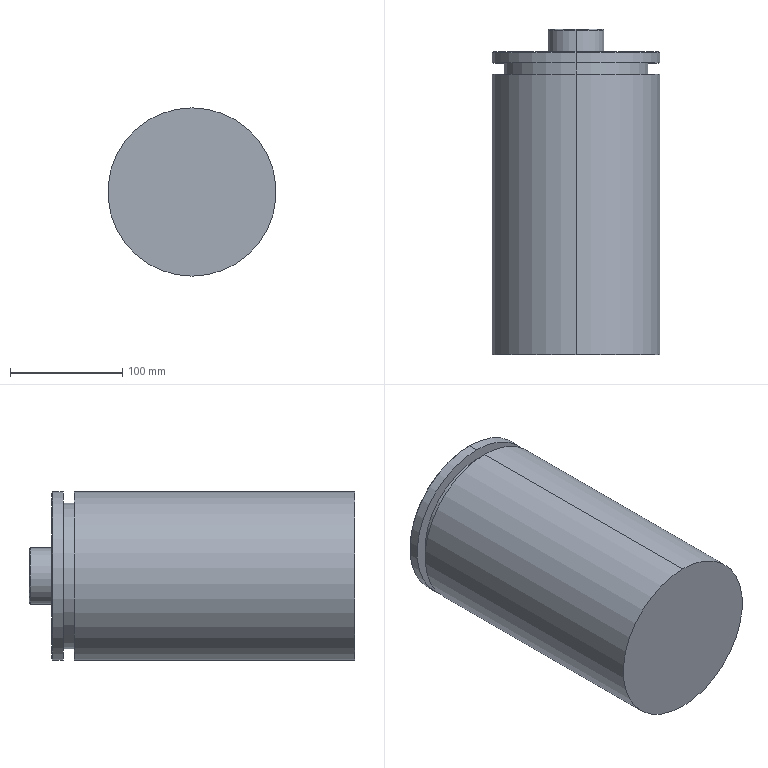Part | SolidWorks | features ICE 3, Chamfer 1, Extrusion 1, Fillet 1 | 1 solid | 17 faces | box 150 x 290 x 150 mm | volume 4766313 mm3 | cylinder 8 | plane 5 | cone 2 | torus 2 | commonest cylinder face diameters 150 x4 50 x2 130 x2
STEP:
#1=CARTESIAN_POINT('',(0.,270.,74.));
#2=VERTEX_POINT('',#1);
#3=CARTESIAN_POINT('',(0.,270.,-74.));
#4=VERTEX_POINT('',#3);
#5=CARTESIAN_POINT('',(0.,270.,0.));
#6=DIRECTION('',(0.,1.,0.));
#7=DIRECTION('',(0.,0.,1.));
#8=AXIS2_PLACEMENT_3D('',#5,#6,#7);
#9=CIRCLE('',#8,74.);
#10=EDGE_CURVE('',#2,#4,#9,.T.);
#11=ORIENTED_EDGE('',*,*,#10,.F.);
#12=CARTESIAN_POINT('',(0.,269.,75.));
#13=VERTEX_POINT('',#12);
#14=CARTESIAN_POINT('',(0.,270.,74.));
#15=DIRECTION('',(0.,-0.7071,0.7071));
#16=VECTOR('',#15,1000.);
#17=LINE('',#14,#16);
#18=EDGE_CURVE('',#2,#13,#17,.T.);
#19=ORIENTED_EDGE('',*,*,#18,.T.);
#20=CARTESIAN_POINT('',(0.,269.,-75.));
#21=VERTEX_POINT('',#20);
#22=CARTESIAN_POINT('',(0.,269.,0.));
#23=DIRECTION('',(0.,-1.,0.));
#24=DIRECTION('',(0.,0.,1.));
#25=AXIS2_PLACEMENT_3D('',#22,#23,#24);
#26=CIRCLE('',#25,75.);
#27=EDGE_CURVE('',#21,#13,#26,.T.);
#28=ORIENTED_EDGE('',*,*,#27,.F.);
#29=CARTESIAN_POINT('',(0.,270.,-74.));
#30=DIRECTION('',(0.,-0.7071,-0.7071));
#31=VECTOR('',#30,1000.);
#32=LINE('',#29,#31);
#33=EDGE_CURVE('',#4,#21,#32,.T.);
#34=ORIENTED_EDGE('',*,*,#33,.F.);
#35=EDGE_LOOP('',(#11,#19,#28,#34));
#36=FACE_OUTER_BOUND('',#35,.T.);
#37=CARTESIAN_POINT('',(0.,270.,0.));
#38=DIRECTION('',(0.,-1.,0.));
#39=DIRECTION('',(0.,0.,-1.));
#40=AXIS2_PLACEMENT_3D('',#37,#38,#39);
#41=CONICAL_SURFACE('',#40,74.,0.7854);
#42=ADVANCED_FACE('',(#36),#41,.T.);
#43=CARTESIAN_POINT('',(0.,289.,-25.));
#44=VERTEX_POINT('',#43);
#45=CARTESIAN_POINT('',(0.,289.,25.));
#46=VERTEX_POINT('',#45);
#47=CARTESIAN_POINT('',(0.,289.,0.));
#48=DIRECTION('',(0.,-1.,0.));
#49=DIRECTION('',(0.,0.,1.));
#50=AXIS2_PLACEMENT_3D('',#47,#48,#49);
#51=CIRCLE('',#50,25.);
#52=EDGE_CURVE('',#44,#46,#51,.T.);
#53=ORIENTED_EDGE('',*,*,#52,.F.);
#54=CARTESIAN_POINT('',(0.,290.,-24.));
#55=VERTEX_POINT('',#54);
#56=CARTESIAN_POINT('',(0.,289.,-24.));
#57=DIRECTION('',(1.,0.,0.));
#58=DIRECTION('',(0.,0.,-1.));
#59=AXIS2_PLACEMENT_3D('',#56,#57,#58);
#60=CIRCLE('',#59,1.);
#61=EDGE_CURVE('',#44,#55,#60,.T.);
#62=ORIENTED_EDGE('',*,*,#61,.T.);
#63=CARTESIAN_POINT('',(0.,290.,24.));
#64=VERTEX_POINT('',#63);
#65=CARTESIAN_POINT('',(0.,290.,0.));
#66=DIRECTION('',(0.,1.,0.));
#67=DIRECTION('',(0.,0.,1.));
#68=AXIS2_PLACEMENT_3D('',#65,#66,#67);
#69=CIRCLE('',#68,24.);
#70=EDGE_CURVE('',#64,#55,#69,.T.);
#71=ORIENTED_EDGE('',*,*,#70,.F.);
#72=CARTESIAN_POINT('',(0.,289.,24.));
#73=DIRECTION('',(-1.,0.,0.));
#74=DIRECTION('',(0.,0.,1.));
#75=AXIS2_PLACEMENT_3D('',#72,#73,#74);
#76=CIRCLE('',#75,1.);
#77=EDGE_CURVE('',#46,#64,#76,.T.);
#78=ORIENTED_EDGE('',*,*,#77,.F.);
#79=EDGE_LOOP('',(#53,#62,#71,#78));
#80=FACE_OUTER_BOUND('',#79,.T.);
#81=CARTESIAN_POINT('',(0.,289.,0.));
#82=DIRECTION('',(0.,1.,0.));
#83=DIRECTION('',(0.,0.,1.));
#84=AXIS2_PLACEMENT_3D('',#81,#82,#83);
#85=TOROIDAL_SURFACE('',#84,24.,1.);
#86=ADVANCED_FACE('',(#80),#85,.T.);
#87=ORIENTED_EDGE('',*,*,#52,.T.);
#88=CARTESIAN_POINT('',(0.,270.,25.));
#89=VERTEX_POINT('',#88);
#90=CARTESIAN_POINT('',(0.,290.,25.));
#91=DIRECTION('',(0.,-1.,0.));
#92=VECTOR('',#91,1000.);
#93=LINE('',#90,#92);
#94=EDGE_CURVE('',#46,#89,#93,.T.);
#95=ORIENTED_EDGE('',*,*,#94,.T.);
#96=CARTESIAN_POINT('',(0.,270.,-25.));
#97=VERTEX_POINT('',#96);
#98=CARTESIAN_POINT('',(0.,270.,0.));
#99=DIRECTION('',(0.,1.,0.));
#100=DIRECTION('',(0.,0.,1.));
#101=AXIS2_PLACEMENT_3D('',#98,#99,#100);
#102=CIRCLE('',#101,25.);
#103=EDGE_CURVE('',#89,#97,#102,.T.);
#104=ORIENTED_EDGE('',*,*,#103,.T.);
#105=CARTESIAN_POINT('',(0.,290.,-25.));
#106=DIRECTION('',(0.,-1.,0.));
#107=VECTOR('',#106,1000.);
#108=LINE('',#105,#107);
#109=EDGE_CURVE('',#44,#97,#108,.T.);
#110=ORIENTED_EDGE('',*,*,#109,.F.);
#111=EDGE_LOOP('',(#87,#95,#104,#110));
#112=FACE_OUTER_BOUND('',#111,.T.);
#113=CARTESIAN_POINT('',(0.,290.,0.));
#114=DIRECTION('',(0.,-1.,0.));
#115=DIRECTION('',(0.,0.,-1.));
#116=AXIS2_PLACEMENT_3D('',#113,#114,#115);
#117=CYLINDRICAL_SURFACE('',#116,25.);
#118=ADVANCED_FACE('',(#112),#117,.T.);
#119=ORIENTED_EDGE('',*,*,#27,.T.);
#120=CARTESIAN_POINT('',(0.,260.,75.));
#121=VERTEX_POINT('',#120);
#122=CARTESIAN_POINT('',(0.,270.,75.));
#123=DIRECTION('',(0.,-1.,0.));
#124=VECTOR('',#123,1000.);
#125=LINE('',#122,#124);
#126=EDGE_CURVE('',#13,#121,#125,.T.);
#127=ORIENTED_EDGE('',*,*,#126,.T.);
#128=CARTESIAN_POINT('',(0.,260.,-75.));
#129=VERTEX_POINT('',#128);
#130=CARTESIAN_POINT('',(0.,260.,0.));
#131=DIRECTION('',(0.,1.,0.));
#132=DIRECTION('',(0.,0.,1.));
#133=AXIS2_PLACEMENT_3D('',#130,#131,#132);
#134=CIRCLE('',#133,75.);
#135=EDGE_CURVE('',#121,#129,#134,.T.);
#136=ORIENTED_EDGE('',*,*,#135,.T.);
#137=CARTESIAN_POINT('',(0.,270.,-75.));
#138=DIRECTION('',(0.,-1.,0.));
#139=VECTOR('',#138,1000.);
#140=LINE('',#137,#139);
#141=EDGE_CURVE('',#21,#129,#140,.T.);
#142=ORIENTED_EDGE('',*,*,#141,.F.);
#143=EDGE_LOOP('',(#119,#127,#136,#142));
#144=FACE_OUTER_BOUND('',#143,.T.);
#145=CARTESIAN_POINT('',(0.,270.,0.));
#146=DIRECTION('',(0.,-1.,0.));
#147=DIRECTION('',(0.,0.,-1.));
#148=AXIS2_PLACEMENT_3D('',#145,#146,#147);
#149=CYLINDRICAL_SURFACE('',#148,75.);
#150=ADVANCED_FACE('',(#144),#149,.T.);
#151=CARTESIAN_POINT('',(0.,260.,65.));
#152=VERTEX_POINT('',#151);
#153=CARTESIAN_POINT('',(0.,260.,-65.));
#154=VERTEX_POINT('',#153);
#155=CARTESIAN_POINT('',(0.,260.,0.));
#156=DIRECTION('',(0.,1.,0.));
#157=DIRECTION('',(0.,0.,1.));
#158=AXIS2_PLACEMENT_3D('',#155,#156,#157);
#159=CIRCLE('',#158,65.);
#160=EDGE_CURVE('',#152,#154,#159,.T.);
#161=ORIENTED_EDGE('',*,*,#160,.F.);
#162=CARTESIAN_POINT('',(0.,250.,65.));
#163=VERTEX_POINT('',#162);
#164=CARTESIAN_POINT('',(0.,260.,65.));
#165=DIRECTION('',(0.,-1.,0.));
#166=VECTOR('',#165,1000.);
#167=LINE('',#164,#166);
#168=EDGE_CURVE('',#152,#163,#167,.T.);
#169=ORIENTED_EDGE('',*,*,#168,.T.);
#170=CARTESIAN_POINT('',(0.,250.,-65.));
#171=VERTEX_POINT('',#170);
#172=CARTESIAN_POINT('',(0.,250.,0.));
#173=DIRECTION('',(0.,1.,0.));
#174=DIRECTION('',(0.,0.,1.));
#175=AXIS2_PLACEMENT_3D('',#172,#173,#174);
#176=CIRCLE('',#175,65.);
#177=EDGE_CURVE('',#163,#171,#176,.T.);
#178=ORIENTED_EDGE('',*,*,#177,.T.);
#179=CARTESIAN_POINT('',(0.,260.,-65.));
#180=DIRECTION('',(0.,-1.,0.));
#181=VECTOR('',#180,1000.);
#182=LINE('',#179,#181);
#183=EDGE_CURVE('',#154,#171,#182,.T.);
#184=ORIENTED_EDGE('',*,*,#183,.F.);
#185=EDGE_LOOP('',(#161,#169,#178,#184));
#186=FACE_OUTER_BOUND('',#185,.T.);
#187=CARTESIAN_POINT('',(0.,260.,0.));
#188=DIRECTION('',(0.,-1.,0.));
#189=DIRECTION('',(0.,0.,-1.));
#190=AXIS2_PLACEMENT_3D('',#187,#188,#189);
#191=CYLINDRICAL_SURFACE('',#190,65.);
#192=ADVANCED_FACE('',(#186),#191,.T.);
#193=CARTESIAN_POINT('',(0.,250.,75.));
#194=VERTEX_POINT('',#193);
#195=CARTESIAN_POINT('',(0.,250.,-75.));
#196=VERTEX_POINT('',#195);
#197=CARTESIAN_POINT('',(0.,250.,0.));
#198=DIRECTION('',(0.,1.,0.));
#199=DIRECTION('',(0.,0.,1.));
#200=AXIS2_PLACEMENT_3D('',#197,#198,#199);
#201=CIRCLE('',#200,75.);
#202=EDGE_CURVE('',#194,#196,#201,.T.);
#203=ORIENTED_EDGE('',*,*,#202,.F.);
#204=CARTESIAN_POINT('',(0.,0.,75.));
#205=VERTEX_POINT('',#204);
#206=CARTESIAN_POINT('',(0.,250.,75.));
#207=DIRECTION('',(0.,-1.,0.));
#208=VECTOR('',#207,1000.);
#209=LINE('',#206,#208);
#210=EDGE_CURVE('',#194,#205,#209,.T.);
#211=ORIENTED_EDGE('',*,*,#210,.T.);
#212=CARTESIAN_POINT('',(0.,0.,-75.));
#213=VERTEX_POINT('',#212);
#214=CARTESIAN_POINT('',(0.,0.,0.));
#215=DIRECTION('',(0.,1.,0.));
#216=DIRECTION('',(0.,0.,1.));
#217=AXIS2_PLACEMENT_3D('',#214,#215,#216);
#218=CIRCLE('',#217,75.);
#219=EDGE_CURVE('',#205,#213,#218,.T.);
#220=ORIENTED_EDGE('',*,*,#219,.T.);
#221=CARTESIAN_POINT('',(0.,250.,-75.));
#222=DIRECTION('',(0.,-1.,0.));
#223=VECTOR('',#222,1000.);
#224=LINE('',#221,#223);
#225=EDGE_CURVE('',#196,#213,#224,.T.);
#226=ORIENTED_EDGE('',*,*,#225,.F.);
#227=EDGE_LOOP('',(#203,#211,#220,#226));
#228=FACE_OUTER_BOUND('',#227,.T.);
#229=CARTESIAN_POINT('',(0.,250.,0.));
#230=DIRECTION('',(0.,-1.,0.));
#231=DIRECTION('',(0.,0.,-1.));
#232=AXIS2_PLACEMENT_3D('',#229,#230,#231);
#233=CYLINDRICAL_SURFACE('',#232,75.);
#234=ADVANCED_FACE('',(#228),#233,.T.);
#235=ORIENTED_EDGE('',*,*,#210,.F.);
#236=CARTESIAN_POINT('',(0.,250.,0.));
#237=DIRECTION('',(0.,1.,0.));
#238=DIRECTION('',(0.,0.,1.));
#239=AXIS2_PLACEMENT_3D('',#236,#237,#238);
#240=CIRCLE('',#239,75.);
#241=EDGE_CURVE('',#196,#194,#240,.T.);
#242=ORIENTED_EDGE('',*,*,#241,.F.);
#243=ORIENTED_EDGE('',*,*,#225,.T.);
#244=CARTESIAN_POINT('',(0.,0.,0.));
#245=DIRECTION('',(0.,1.,0.));
#246=DIRECTION('',(0.,0.,1.));
#247=AXIS2_PLACEMENT_3D('',#244,#245,#246);
#248=CIRCLE('',#247,75.);
#249=EDGE_CURVE('',#213,#205,#248,.T.);
#250=ORIENTED_EDGE('',*,*,#249,.T.);
#251=EDGE_LOOP('',(#235,#242,#243,#250));
#252=FACE_OUTER_BOUND('',#251,.T.);
#253=CARTESIAN_POINT('',(0.,250.,0.));
#254=DIRECTION('',(0.,-1.,0.));
#255=DIRECTION('',(0.,0.,-1.));
#256=AXIS2_PLACEMENT_3D('',#253,#254,#255);
#257=CYLINDRICAL_SURFACE('',#256,75.);
#258=ADVANCED_FACE('',(#252),#257,.T.);
#259=CARTESIAN_POINT('',(0.,250.,0.));
#260=DIRECTION('',(0.,1.,0.));
#261=DIRECTION('',(0.,0.,1.));
#262=AXIS2_PLACEMENT_3D('',#259,#260,#261);
#263=CIRCLE('',#262,65.);
#264=EDGE_CURVE('',#171,#163,#263,.T.);
#265=ORIENTED_EDGE('',*,*,#264,.F.);
#266=ORIENTED_EDGE('',*,*,#177,.F.);
#267=EDGE_LOOP('',(#265,#266));
#268=FACE_BOUND('',#267,.T.);
#269=ORIENTED_EDGE('',*,*,#241,.T.);
#270=ORIENTED_EDGE('',*,*,#202,.T.);
#271=EDGE_LOOP('',(#269,#270));
#272=FACE_OUTER_BOUND('',#271,.T.);
#273=CARTESIAN_POINT('',(0.,250.,0.));
#274=DIRECTION('',(0.,1.,0.));
#275=DIRECTION('',(0.,0.,1.));
#276=AXIS2_PLACEMENT_3D('',#273,#274,#275);
#277=PLANE('',#276);
#278=ADVANCED_FACE('',(#268,#272),#277,.T.);
#279=ORIENTED_EDGE('',*,*,#249,.F.);
#280=ORIENTED_EDGE('',*,*,#219,.F.);
#281=EDGE_LOOP('',(#279,#280));
#282=FACE_OUTER_BOUND('',#281,.T.);
#283=CARTESIAN_POINT('',(0.,0.,0.));
#284=DIRECTION('',(0.,1.,0.));
#285=DIRECTION('',(0.,0.,1.));
#286=AXIS2_PLACEMENT_3D('',#283,#284,#285);
#287=PLANE('',#286);
#288=ADVANCED_FACE('',(#282),#287,.F.);
#289=ORIENTED_EDGE('',*,*,#168,.F.);
#290=CARTESIAN_POINT('',(0.,260.,0.));
#291=DIRECTION('',(0.,1.,0.));
#292=DIRECTION('',(0.,0.,1.));
#293=AXIS2_PLACEMENT_3D('',#290,#291,#292);
#294=CIRCLE('',#293,65.);
#295=EDGE_CURVE('',#154,#152,#294,.T.);
#296=ORIENTED_EDGE('',*,*,#295,.F.);
#297=ORIENTED_EDGE('',*,*,#183,.T.);
#298=ORIENTED_EDGE('',*,*,#264,.T.);
#299=EDGE_LOOP('',(#289,#296,#297,#298));
#300=FACE_OUTER_BOUND('',#299,.T.);
#301=CARTESIAN_POINT('',(0.,260.,0.));
#302=DIRECTION('',(0.,-1.,0.));
#303=DIRECTION('',(0.,0.,-1.));
#304=AXIS2_PLACEMENT_3D('',#301,#302,#303);
#305=CYLINDRICAL_SURFACE('',#304,65.);
#306=ADVANCED_FACE('',(#300),#305,.T.);
#307=ORIENTED_EDGE('',*,*,#126,.F.);
#308=CARTESIAN_POINT('',(0.,269.,0.));
#309=DIRECTION('',(0.,-1.,0.));
#310=DIRECTION('',(0.,0.,1.));
#311=AXIS2_PLACEMENT_3D('',#308,#309,#310);
#312=CIRCLE('',#311,75.);
#313=EDGE_CURVE('',#13,#21,#312,.T.);
#314=ORIENTED_EDGE('',*,*,#313,.T.);
#315=ORIENTED_EDGE('',*,*,#141,.T.);
#316=CARTESIAN_POINT('',(0.,260.,0.));
#317=DIRECTION('',(0.,1.,0.));
#318=DIRECTION('',(0.,0.,1.));
#319=AXIS2_PLACEMENT_3D('',#316,#317,#318);
#320=CIRCLE('',#319,75.);
#321=EDGE_CURVE('',#129,#121,#320,.T.);
#322=ORIENTED_EDGE('',*,*,#321,.T.);
#323=EDGE_LOOP('',(#307,#314,#315,#322));
#324=FACE_OUTER_BOUND('',#323,.T.);
#325=CARTESIAN_POINT('',(0.,270.,0.));
#326=DIRECTION('',(0.,-1.,0.));
#327=DIRECTION('',(0.,0.,-1.));
#328=AXIS2_PLACEMENT_3D('',#325,#326,#327);
#329=CYLINDRICAL_SURFACE('',#328,75.);
#330=ADVANCED_FACE('',(#324),#329,.T.);
#331=CARTESIAN_POINT('',(0.,270.,0.));
#332=DIRECTION('',(0.,1.,0.));
#333=DIRECTION('',(0.,0.,1.));
#334=AXIS2_PLACEMENT_3D('',#331,#332,#333);
#335=CIRCLE('',#334,74.);
#336=EDGE_CURVE('',#4,#2,#335,.T.);
#337=ORIENTED_EDGE('',*,*,#336,.T.);
#338=ORIENTED_EDGE('',*,*,#10,.T.);
#339=EDGE_LOOP('',(#337,#338));
#340=FACE_OUTER_BOUND('',#339,.T.);
#341=CARTESIAN_POINT('',(0.,270.,0.));
#342=DIRECTION('',(0.,1.,0.));
#343=DIRECTION('',(0.,0.,1.));
#344=AXIS2_PLACEMENT_3D('',#341,#342,#343);
#345=CIRCLE('',#344,25.);
#346=EDGE_CURVE('',#97,#89,#345,.T.);
#347=ORIENTED_EDGE('',*,*,#346,.F.);
#348=ORIENTED_EDGE('',*,*,#103,.F.);
#349=EDGE_LOOP('',(#347,#348));
#350=FACE_BOUND('',#349,.T.);
#351=CARTESIAN_POINT('',(0.,270.,0.));
#352=DIRECTION('',(0.,1.,0.));
#353=DIRECTION('',(0.,0.,1.));
#354=AXIS2_PLACEMENT_3D('',#351,#352,#353);
#355=PLANE('',#354);
#356=ADVANCED_FACE('',(#340,#350),#355,.T.);
#357=ORIENTED_EDGE('',*,*,#295,.T.);
#358=ORIENTED_EDGE('',*,*,#160,.T.);
#359=EDGE_LOOP('',(#357,#358));
#360=FACE_BOUND('',#359,.T.);
#361=ORIENTED_EDGE('',*,*,#321,.F.);
#362=ORIENTED_EDGE('',*,*,#135,.F.);
#363=EDGE_LOOP('',(#361,#362));
#364=FACE_OUTER_BOUND('',#363,.T.);
#365=CARTESIAN_POINT('',(0.,260.,0.));
#366=DIRECTION('',(0.,1.,0.));
#367=DIRECTION('',(0.,0.,1.));
#368=AXIS2_PLACEMENT_3D('',#365,#366,#367);
#369=PLANE('',#368);
#370=ADVANCED_FACE('',(#360,#364),#369,.F.);
#371=ORIENTED_EDGE('',*,*,#94,.F.);
#372=CARTESIAN_POINT('',(0.,289.,0.));
#373=DIRECTION('',(0.,-1.,0.));
#374=DIRECTION('',(0.,0.,1.));
#375=AXIS2_PLACEMENT_3D('',#372,#373,#374);
#376=CIRCLE('',#375,25.);
#377=EDGE_CURVE('',#46,#44,#376,.T.);
#378=ORIENTED_EDGE('',*,*,#377,.T.);
#379=ORIENTED_EDGE('',*,*,#109,.T.);
#380=ORIENTED_EDGE('',*,*,#346,.T.);
#381=EDGE_LOOP('',(#371,#378,#379,#380));
#382=FACE_OUTER_BOUND('',#381,.T.);
#383=CARTESIAN_POINT('',(0.,290.,0.));
#384=DIRECTION('',(0.,-1.,0.));
#385=DIRECTION('',(0.,0.,-1.));
#386=AXIS2_PLACEMENT_3D('',#383,#384,#385);
#387=CYLINDRICAL_SURFACE('',#386,25.);
#388=ADVANCED_FACE('',(#382),#387,.T.);
#389=ORIENTED_EDGE('',*,*,#70,.T.);
#390=CARTESIAN_POINT('',(0.,290.,0.));
#391=DIRECTION('',(0.,1.,0.));
#392=DIRECTION('',(0.,0.,1.));
#393=AXIS2_PLACEMENT_3D('',#390,#391,#392);
#394=CIRCLE('',#393,24.);
#395=EDGE_CURVE('',#55,#64,#394,.T.);
#396=ORIENTED_EDGE('',*,*,#395,.T.);
#397=EDGE_LOOP('',(#389,#396));
#398=FACE_OUTER_BOUND('',#397,.T.);
#399=CARTESIAN_POINT('',(0.,290.,0.));
#400=DIRECTION('',(0.,1.,0.));
#401=DIRECTION('',(0.,0.,1.));
#402=AXIS2_PLACEMENT_3D('',#399,#400,#401);
#403=PLANE('',#402);
#404=ADVANCED_FACE('',(#398),#403,.T.);
#405=ORIENTED_EDGE('',*,*,#61,.F.);
#406=ORIENTED_EDGE('',*,*,#377,.F.);
#407=ORIENTED_EDGE('',*,*,#77,.T.);
#408=ORIENTED_EDGE('',*,*,#395,.F.);
#409=EDGE_LOOP('',(#405,#406,#407,#408));
#410=FACE_OUTER_BOUND('',#409,.T.);
#411=CARTESIAN_POINT('',(0.,289.,0.));
#412=DIRECTION('',(0.,1.,0.));
#413=DIRECTION('',(0.,0.,1.));
#414=AXIS2_PLACEMENT_3D('',#411,#412,#413);
#415=TOROIDAL_SURFACE('',#414,24.,1.);
#416=ADVANCED_FACE('',(#410),#415,.T.);
#417=ORIENTED_EDGE('',*,*,#18,.F.);
#418=ORIENTED_EDGE('',*,*,#336,.F.);
#419=ORIENTED_EDGE('',*,*,#33,.T.);
#420=ORIENTED_EDGE('',*,*,#313,.F.);
#421=EDGE_LOOP('',(#417,#418,#419,#420));
#422=FACE_OUTER_BOUND('',#421,.T.);
#423=CARTESIAN_POINT('',(0.,270.,0.));
#424=DIRECTION('',(0.,-1.,0.));
#425=DIRECTION('',(0.,0.,-1.));
#426=AXIS2_PLACEMENT_3D('',#423,#424,#425);
#427=CONICAL_SURFACE('',#426,74.,0.7854);
#428=ADVANCED_FACE('',(#422),#427,.T.);
#429=CLOSED_SHELL('',(#42,#86,#118,#150,#192,#234,#258,#278,#288,#306,#330,#356,#370,#388,#404,#416,#428));
#430=MANIFOLD_SOLID_BREP('',#429);
#431=CARTESIAN_POINT('',(0.,0.,0.));
#432=DIRECTION('',(0.,0.,1.));
#433=DIRECTION('',(1.,0.,0.));
#434=AXIS2_PLACEMENT_3D('',#431,#432,#433);
#435=(LENGTH_UNIT()NAMED_UNIT(*)SI_UNIT(.MILLI.,.METRE.));
#436=UNCERTAINTY_MEASURE_WITH_UNIT(LENGTH_MEASURE(0.00001),#435,'','');
#437=(NAMED_UNIT(*)PLANE_ANGLE_UNIT()SI_UNIT($,.RADIAN.));
#438=(NAMED_UNIT(*)SI_UNIT($,.STERADIAN.)SOLID_ANGLE_UNIT());
#439=(GEOMETRIC_REPRESENTATION_CONTEXT(3)GLOBAL_UNCERTAINTY_ASSIGNED_CONTEXT((#436))GLOBAL_UNIT_ASSIGNED_CONTEXT((#435,#437,#438))REPRESENTATION_CONTEXT('',''));
#440=ADVANCED_BREP_SHAPE_REPRESENTATION('',(#430,#434),#439);